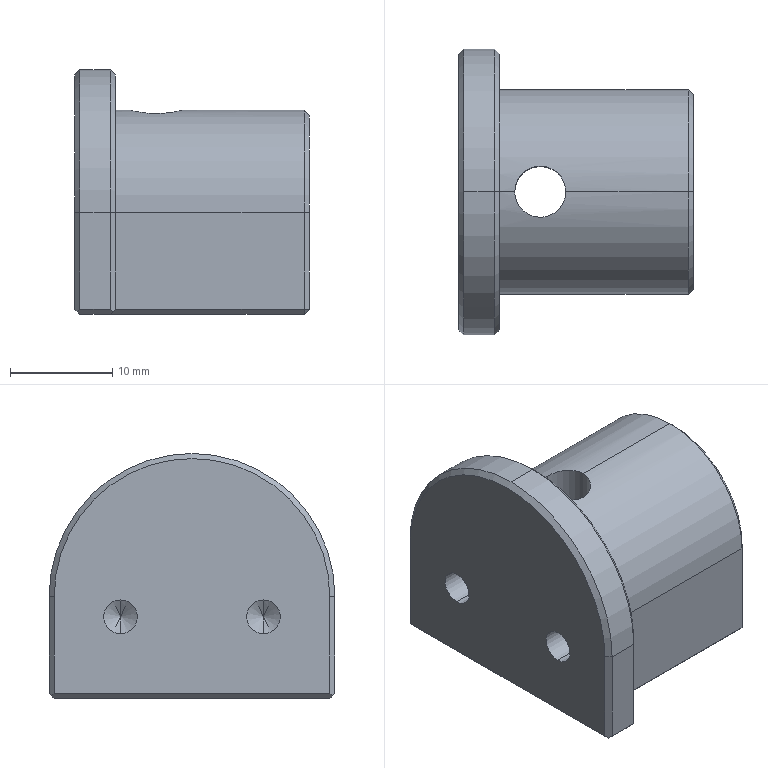Part | STEP file | PN_0014 driven wheel fixing block_Default | 1 solid | 47 faces | box 23 x 28 x 24 mm | volume 8364 mm3 | plane 24 | cylinder 12 | cone 11 | commonest cylinder face diameters 3.3 x4 4.2 x2 5 x2 20 x2 28 x2